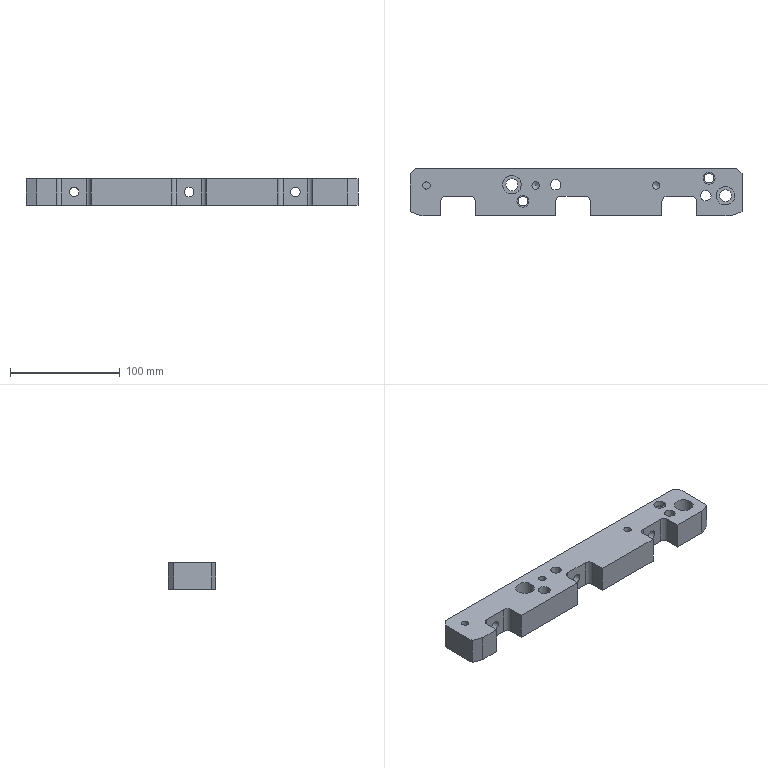Part | STEP file | 1_id1118_x_t | 1 solid | 63 faces | box 303 x 43.296 x 24.5 mm | volume 252825 mm3 | plane 32 | cylinder 27 | cone 4 | commonest cylinder face diameters 9.525 x4 11 x4 6.75 x3 8.7 x3 15 x3 8 x2